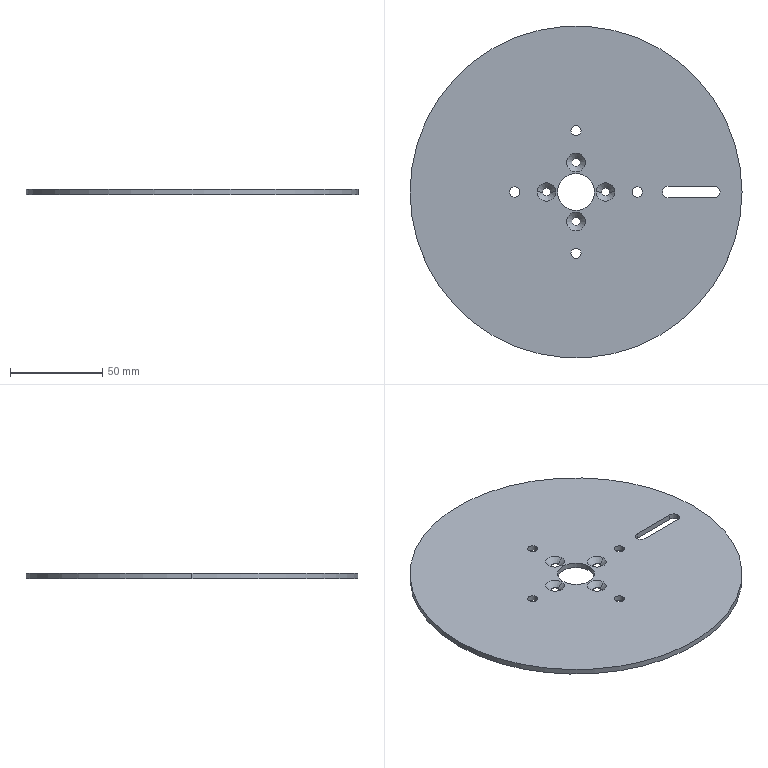Part | SolidWorks | features Chamfer 1, Extrusion 1, ICE 1 | 1 solid | 35 faces | box 180 x 180 x 3 mm | volume 74053 mm3 | cylinder 23 | cone 8 | plane 4 | commonest cylinder face diameters 4.5 x8 5.5 x8 6.2 x3 20 x2 180 x2
STEP:
#1=CARTESIAN_POINT('',(-18.25,0.,0.2));
#2=VERTEX_POINT('',#1);
#3=CARTESIAN_POINT('',(-13.75,0.,0.2));
#4=VERTEX_POINT('',#3);
#5=CARTESIAN_POINT('',(-16.,0.,0.2));
#6=DIRECTION('',(0.,0.,1.));
#7=DIRECTION('',(1.,0.,0.));
#8=AXIS2_PLACEMENT_3D('',#5,#6,#7);
#9=CIRCLE('',#8,2.25);
#10=EDGE_CURVE('',#2,#4,#9,.T.);
#11=ORIENTED_EDGE('',*,*,#10,.F.);
#12=CARTESIAN_POINT('',(-21.05,0.,3.));
#13=VERTEX_POINT('',#12);
#14=CARTESIAN_POINT('',(-18.25,0.,0.2));
#15=DIRECTION('',(-0.7071,0.,0.7071));
#16=VECTOR('',#15,1000.);
#17=LINE('',#14,#16);
#18=EDGE_CURVE('',#2,#13,#17,.T.);
#19=ORIENTED_EDGE('',*,*,#18,.T.);
#20=CARTESIAN_POINT('',(-10.95,0.,3.));
#21=VERTEX_POINT('',#20);
#22=CARTESIAN_POINT('',(-16.,0.,3.));
#23=DIRECTION('',(0.,0.,-1.));
#24=DIRECTION('',(1.,0.,0.));
#25=AXIS2_PLACEMENT_3D('',#22,#23,#24);
#26=CIRCLE('',#25,5.05);
#27=EDGE_CURVE('',#21,#13,#26,.T.);
#28=ORIENTED_EDGE('',*,*,#27,.F.);
#29=CARTESIAN_POINT('',(-13.75,0.,0.2));
#30=DIRECTION('',(0.7071,0.,0.7071));
#31=VECTOR('',#30,1000.);
#32=LINE('',#29,#31);
#33=EDGE_CURVE('',#4,#21,#32,.T.);
#34=ORIENTED_EDGE('',*,*,#33,.F.);
#35=EDGE_LOOP('',(#11,#19,#28,#34));
#36=FACE_OUTER_BOUND('',#35,.T.);
#37=CARTESIAN_POINT('',(-16.,0.,0.2));
#38=DIRECTION('',(0.,0.,1.));
#39=DIRECTION('',(1.,0.,0.));
#40=AXIS2_PLACEMENT_3D('',#37,#38,#39);
#41=CONICAL_SURFACE('',#40,2.25,0.7854);
#42=ADVANCED_FACE('',(#36),#41,.F.);
#43=CARTESIAN_POINT('',(-2.25,16.,0.2));
#44=VERTEX_POINT('',#43);
#45=CARTESIAN_POINT('',(2.25,16.,0.2));
#46=VERTEX_POINT('',#45);
#47=CARTESIAN_POINT('',(0.,16.,0.2));
#48=DIRECTION('',(0.,0.,1.));
#49=DIRECTION('',(1.,0.,0.));
#50=AXIS2_PLACEMENT_3D('',#47,#48,#49);
#51=CIRCLE('',#50,2.25);
#52=EDGE_CURVE('',#44,#46,#51,.T.);
#53=ORIENTED_EDGE('',*,*,#52,.F.);
#54=CARTESIAN_POINT('',(-5.05,16.,3.));
#55=VERTEX_POINT('',#54);
#56=CARTESIAN_POINT('',(-2.25,16.,0.2));
#57=DIRECTION('',(-0.7071,0.,0.7071));
#58=VECTOR('',#57,1000.);
#59=LINE('',#56,#58);
#60=EDGE_CURVE('',#44,#55,#59,.T.);
#61=ORIENTED_EDGE('',*,*,#60,.T.);
#62=CARTESIAN_POINT('',(5.05,16.,3.));
#63=VERTEX_POINT('',#62);
#64=CARTESIAN_POINT('',(0.,16.,3.));
#65=DIRECTION('',(0.,0.,-1.));
#66=DIRECTION('',(1.,0.,0.));
#67=AXIS2_PLACEMENT_3D('',#64,#65,#66);
#68=CIRCLE('',#67,5.05);
#69=EDGE_CURVE('',#63,#55,#68,.T.);
#70=ORIENTED_EDGE('',*,*,#69,.F.);
#71=CARTESIAN_POINT('',(2.25,16.,0.2));
#72=DIRECTION('',(0.7071,0.,0.7071));
#73=VECTOR('',#72,1000.);
#74=LINE('',#71,#73);
#75=EDGE_CURVE('',#46,#63,#74,.T.);
#76=ORIENTED_EDGE('',*,*,#75,.F.);
#77=EDGE_LOOP('',(#53,#61,#70,#76));
#78=FACE_OUTER_BOUND('',#77,.T.);
#79=CARTESIAN_POINT('',(0.,16.,0.2));
#80=DIRECTION('',(0.,0.,1.));
#81=DIRECTION('',(1.,0.,0.));
#82=AXIS2_PLACEMENT_3D('',#79,#80,#81);
#83=CONICAL_SURFACE('',#82,2.25,0.7854);
#84=ADVANCED_FACE('',(#78),#83,.F.);
#85=CARTESIAN_POINT('',(13.75,0.,0.2));
#86=VERTEX_POINT('',#85);
#87=CARTESIAN_POINT('',(18.25,0.,0.2));
#88=VERTEX_POINT('',#87);
#89=CARTESIAN_POINT('',(16.,0.,0.2));
#90=DIRECTION('',(0.,0.,1.));
#91=DIRECTION('',(1.,0.,0.));
#92=AXIS2_PLACEMENT_3D('',#89,#90,#91);
#93=CIRCLE('',#92,2.25);
#94=EDGE_CURVE('',#86,#88,#93,.T.);
#95=ORIENTED_EDGE('',*,*,#94,.F.);
#96=CARTESIAN_POINT('',(10.95,0.,3.));
#97=VERTEX_POINT('',#96);
#98=CARTESIAN_POINT('',(13.75,0.,0.2));
#99=DIRECTION('',(-0.7071,0.,0.7071));
#100=VECTOR('',#99,1000.);
#101=LINE('',#98,#100);
#102=EDGE_CURVE('',#86,#97,#101,.T.);
#103=ORIENTED_EDGE('',*,*,#102,.T.);
#104=CARTESIAN_POINT('',(21.05,0.,3.));
#105=VERTEX_POINT('',#104);
#106=CARTESIAN_POINT('',(16.,0.,3.));
#107=DIRECTION('',(0.,0.,-1.));
#108=DIRECTION('',(1.,0.,0.));
#109=AXIS2_PLACEMENT_3D('',#106,#107,#108);
#110=CIRCLE('',#109,5.05);
#111=EDGE_CURVE('',#105,#97,#110,.T.);
#112=ORIENTED_EDGE('',*,*,#111,.F.);
#113=CARTESIAN_POINT('',(18.25,0.,0.2));
#114=DIRECTION('',(0.7071,0.,0.7071));
#115=VECTOR('',#114,1000.);
#116=LINE('',#113,#115);
#117=EDGE_CURVE('',#88,#105,#116,.T.);
#118=ORIENTED_EDGE('',*,*,#117,.F.);
#119=EDGE_LOOP('',(#95,#103,#112,#118));
#120=FACE_OUTER_BOUND('',#119,.T.);
#121=CARTESIAN_POINT('',(16.,0.,0.2));
#122=DIRECTION('',(0.,0.,1.));
#123=DIRECTION('',(1.,0.,0.));
#124=AXIS2_PLACEMENT_3D('',#121,#122,#123);
#125=CONICAL_SURFACE('',#124,2.25,0.7854);
#126=ADVANCED_FACE('',(#120),#125,.F.);
#127=CARTESIAN_POINT('',(-2.25,-16.,0.2));
#128=VERTEX_POINT('',#127);
#129=CARTESIAN_POINT('',(2.25,-16.,0.2));
#130=VERTEX_POINT('',#129);
#131=CARTESIAN_POINT('',(0.,-16.,0.2));
#132=DIRECTION('',(0.,0.,1.));
#133=DIRECTION('',(1.,0.,0.));
#134=AXIS2_PLACEMENT_3D('',#131,#132,#133);
#135=CIRCLE('',#134,2.25);
#136=EDGE_CURVE('',#128,#130,#135,.T.);
#137=ORIENTED_EDGE('',*,*,#136,.F.);
#138=CARTESIAN_POINT('',(-5.05,-16.,3.));
#139=VERTEX_POINT('',#138);
#140=CARTESIAN_POINT('',(-2.25,-16.,0.2));
#141=DIRECTION('',(-0.7071,0.,0.7071));
#142=VECTOR('',#141,1000.);
#143=LINE('',#140,#142);
#144=EDGE_CURVE('',#128,#139,#143,.T.);
#145=ORIENTED_EDGE('',*,*,#144,.T.);
#146=CARTESIAN_POINT('',(5.05,-16.,3.));
#147=VERTEX_POINT('',#146);
#148=CARTESIAN_POINT('',(0.,-16.,3.));
#149=DIRECTION('',(0.,0.,-1.));
#150=DIRECTION('',(1.,0.,0.));
#151=AXIS2_PLACEMENT_3D('',#148,#149,#150);
#152=CIRCLE('',#151,5.05);
#153=EDGE_CURVE('',#147,#139,#152,.T.);
#154=ORIENTED_EDGE('',*,*,#153,.F.);
#155=CARTESIAN_POINT('',(2.25,-16.,0.2));
#156=DIRECTION('',(0.7071,0.,0.7071));
#157=VECTOR('',#156,1000.);
#158=LINE('',#155,#157);
#159=EDGE_CURVE('',#130,#147,#158,.T.);
#160=ORIENTED_EDGE('',*,*,#159,.F.);
#161=EDGE_LOOP('',(#137,#145,#154,#160));
#162=FACE_OUTER_BOUND('',#161,.T.);
#163=CARTESIAN_POINT('',(0.,-16.,0.2));
#164=DIRECTION('',(0.,0.,1.));
#165=DIRECTION('',(1.,0.,0.));
#166=AXIS2_PLACEMENT_3D('',#163,#164,#165);
#167=CONICAL_SURFACE('',#166,2.25,0.7854);
#168=ADVANCED_FACE('',(#162),#167,.F.);
#169=CARTESIAN_POINT('',(78.1,0.,0.));
#170=VERTEX_POINT('',#169);
#171=CARTESIAN_POINT('',(75.,3.1,0.));
#172=VERTEX_POINT('',#171);
#173=CARTESIAN_POINT('',(75.,0.,0.));
#174=DIRECTION('',(0.,0.,1.));
#175=DIRECTION('',(1.,0.,0.));
#176=AXIS2_PLACEMENT_3D('',#173,#174,#175);
#177=CIRCLE('',#176,3.1);
#178=EDGE_CURVE('',#170,#172,#177,.T.);
#179=ORIENTED_EDGE('',*,*,#178,.F.);
#180=CARTESIAN_POINT('',(78.1,0.,3.));
#181=VERTEX_POINT('',#180);
#182=CARTESIAN_POINT('',(78.1,0.,0.));
#183=DIRECTION('',(0.,0.,1.));
#184=VECTOR('',#183,1000.);
#185=LINE('',#182,#184);
#186=EDGE_CURVE('',#170,#181,#185,.T.);
#187=ORIENTED_EDGE('',*,*,#186,.T.);
#188=CARTESIAN_POINT('',(75.,3.1,3.));
#189=VERTEX_POINT('',#188);
#190=CARTESIAN_POINT('',(75.,0.,3.));
#191=DIRECTION('',(0.,0.,1.));
#192=DIRECTION('',(1.,0.,0.));
#193=AXIS2_PLACEMENT_3D('',#190,#191,#192);
#194=CIRCLE('',#193,3.1);
#195=EDGE_CURVE('',#181,#189,#194,.T.);
#196=ORIENTED_EDGE('',*,*,#195,.T.);
#197=CARTESIAN_POINT('',(75.,3.1,0.));
#198=DIRECTION('',(0.,0.,1.));
#199=VECTOR('',#198,1000.);
#200=LINE('',#197,#199);
#201=EDGE_CURVE('',#172,#189,#200,.T.);
#202=ORIENTED_EDGE('',*,*,#201,.F.);
#203=EDGE_LOOP('',(#179,#187,#196,#202));
#204=FACE_OUTER_BOUND('',#203,.T.);
#205=CARTESIAN_POINT('',(75.,0.,0.));
#206=DIRECTION('',(0.,0.,1.));
#207=DIRECTION('',(1.,0.,0.));
#208=AXIS2_PLACEMENT_3D('',#205,#206,#207);
#209=CYLINDRICAL_SURFACE('',#208,3.1);
#210=ADVANCED_FACE('',(#204),#209,.F.);
#211=CARTESIAN_POINT('',(30.5,0.,0.));
#212=VERTEX_POINT('',#211);
#213=CARTESIAN_POINT('',(36.,0.,0.));
#214=VERTEX_POINT('',#213);
#215=CARTESIAN_POINT('',(33.25,0.,0.));
#216=DIRECTION('',(0.,0.,1.));
#217=DIRECTION('',(1.,0.,0.));
#218=AXIS2_PLACEMENT_3D('',#215,#216,#217);
#219=CIRCLE('',#218,2.75);
#220=EDGE_CURVE('',#212,#214,#219,.T.);
#221=ORIENTED_EDGE('',*,*,#220,.F.);
#222=CARTESIAN_POINT('',(30.5,0.,3.));
#223=VERTEX_POINT('',#222);
#224=CARTESIAN_POINT('',(30.5,0.,0.));
#225=DIRECTION('',(0.,0.,1.));
#226=VECTOR('',#225,1000.);
#227=LINE('',#224,#226);
#228=EDGE_CURVE('',#212,#223,#227,.T.);
#229=ORIENTED_EDGE('',*,*,#228,.T.);
#230=CARTESIAN_POINT('',(36.,0.,3.));
#231=VERTEX_POINT('',#230);
#232=CARTESIAN_POINT('',(33.25,0.,3.));
#233=DIRECTION('',(0.,0.,1.));
#234=DIRECTION('',(1.,0.,0.));
#235=AXIS2_PLACEMENT_3D('',#232,#233,#234);
#236=CIRCLE('',#235,2.75);
#237=EDGE_CURVE('',#223,#231,#236,.T.);
#238=ORIENTED_EDGE('',*,*,#237,.T.);
#239=CARTESIAN_POINT('',(36.,0.,0.));
#240=DIRECTION('',(0.,0.,1.));
#241=VECTOR('',#240,1000.);
#242=LINE('',#239,#241);
#243=EDGE_CURVE('',#214,#231,#242,.T.);
#244=ORIENTED_EDGE('',*,*,#243,.F.);
#245=EDGE_LOOP('',(#221,#229,#238,#244));
#246=FACE_OUTER_BOUND('',#245,.T.);
#247=CARTESIAN_POINT('',(33.25,0.,0.));
#248=DIRECTION('',(0.,0.,1.));
#249=DIRECTION('',(1.,0.,0.));
#250=AXIS2_PLACEMENT_3D('',#247,#248,#249);
#251=CYLINDRICAL_SURFACE('',#250,2.75);
#252=ADVANCED_FACE('',(#246),#251,.F.);
#253=CARTESIAN_POINT('',(-2.75,-33.25,0.));
#254=VERTEX_POINT('',#253);
#255=CARTESIAN_POINT('',(2.75,-33.25,0.));
#256=VERTEX_POINT('',#255);
#257=CARTESIAN_POINT('',(0.,-33.25,0.));
#258=DIRECTION('',(0.,0.,1.));
#259=DIRECTION('',(1.,0.,0.));
#260=AXIS2_PLACEMENT_3D('',#257,#258,#259);
#261=CIRCLE('',#260,2.75);
#262=EDGE_CURVE('',#254,#256,#261,.T.);
#263=ORIENTED_EDGE('',*,*,#262,.F.);
#264=CARTESIAN_POINT('',(-2.75,-33.25,3.));
#265=VERTEX_POINT('',#264);
#266=CARTESIAN_POINT('',(-2.75,-33.25,0.));
#267=DIRECTION('',(0.,0.,1.));
#268=VECTOR('',#267,1000.);
#269=LINE('',#266,#268);
#270=EDGE_CURVE('',#254,#265,#269,.T.);
#271=ORIENTED_EDGE('',*,*,#270,.T.);
#272=CARTESIAN_POINT('',(2.75,-33.25,3.));
#273=VERTEX_POINT('',#272);
#274=CARTESIAN_POINT('',(0.,-33.25,3.));
#275=DIRECTION('',(0.,0.,1.));
#276=DIRECTION('',(1.,0.,0.));
#277=AXIS2_PLACEMENT_3D('',#274,#275,#276);
#278=CIRCLE('',#277,2.75);
#279=EDGE_CURVE('',#265,#273,#278,.T.);
#280=ORIENTED_EDGE('',*,*,#279,.T.);
#281=CARTESIAN_POINT('',(2.75,-33.25,0.));
#282=DIRECTION('',(0.,0.,1.));
#283=VECTOR('',#282,1000.);
#284=LINE('',#281,#283);
#285=EDGE_CURVE('',#256,#273,#284,.T.);
#286=ORIENTED_EDGE('',*,*,#285,.F.);
#287=EDGE_LOOP('',(#263,#271,#280,#286));
#288=FACE_OUTER_BOUND('',#287,.T.);
#289=CARTESIAN_POINT('',(0.,-33.25,0.));
#290=DIRECTION('',(0.,0.,1.));
#291=DIRECTION('',(1.,0.,0.));
#292=AXIS2_PLACEMENT_3D('',#289,#290,#291);
#293=CYLINDRICAL_SURFACE('',#292,2.75);
#294=ADVANCED_FACE('',(#288),#293,.F.);
#295=CARTESIAN_POINT('',(-36.,0.,0.));
#296=VERTEX_POINT('',#295);
#297=CARTESIAN_POINT('',(-30.5,0.,0.));
#298=VERTEX_POINT('',#297);
#299=CARTESIAN_POINT('',(-33.25,0.,0.));
#300=DIRECTION('',(0.,0.,1.));
#301=DIRECTION('',(1.,0.,0.));
#302=AXIS2_PLACEMENT_3D('',#299,#300,#301);
#303=CIRCLE('',#302,2.75);
#304=EDGE_CURVE('',#296,#298,#303,.T.);
#305=ORIENTED_EDGE('',*,*,#304,.F.);
#306=CARTESIAN_POINT('',(-36.,0.,3.));
#307=VERTEX_POINT('',#306);
#308=CARTESIAN_POINT('',(-36.,0.,0.));
#309=DIRECTION('',(0.,0.,1.));
#310=VECTOR('',#309,1000.);
#311=LINE('',#308,#310);
#312=EDGE_CURVE('',#296,#307,#311,.T.);
#313=ORIENTED_EDGE('',*,*,#312,.T.);
#314=CARTESIAN_POINT('',(-30.5,0.,3.));
#315=VERTEX_POINT('',#314);
#316=CARTESIAN_POINT('',(-33.25,0.,3.));
#317=DIRECTION('',(0.,0.,1.));
#318=DIRECTION('',(1.,0.,0.));
#319=AXIS2_PLACEMENT_3D('',#316,#317,#318);
#320=CIRCLE('',#319,2.75);
#321=EDGE_CURVE('',#307,#315,#320,.T.);
#322=ORIENTED_EDGE('',*,*,#321,.T.);
#323=CARTESIAN_POINT('',(-30.5,0.,0.));
#324=DIRECTION('',(0.,0.,1.));
#325=VECTOR('',#324,1000.);
#326=LINE('',#323,#325);
#327=EDGE_CURVE('',#298,#315,#326,.T.);
#328=ORIENTED_EDGE('',*,*,#327,.F.);
#329=EDGE_LOOP('',(#305,#313,#322,#328));
#330=FACE_OUTER_BOUND('',#329,.T.);
#331=CARTESIAN_POINT('',(-33.25,0.,0.));
#332=DIRECTION('',(0.,0.,1.));
#333=DIRECTION('',(1.,0.,0.));
#334=AXIS2_PLACEMENT_3D('',#331,#332,#333);
#335=CYLINDRICAL_SURFACE('',#334,2.75);
#336=ADVANCED_FACE('',(#330),#335,.F.);
#337=CARTESIAN_POINT('',(-2.75,33.25,0.));
#338=VERTEX_POINT('',#337);
#339=CARTESIAN_POINT('',(2.75,33.25,0.));
#340=VERTEX_POINT('',#339);
#341=CARTESIAN_POINT('',(0.,33.25,0.));
#342=DIRECTION('',(0.,0.,1.));
#343=DIRECTION('',(1.,0.,0.));
#344=AXIS2_PLACEMENT_3D('',#341,#342,#343);
#345=CIRCLE('',#344,2.75);
#346=EDGE_CURVE('',#338,#340,#345,.T.);
#347=ORIENTED_EDGE('',*,*,#346,.F.);
#348=CARTESIAN_POINT('',(-2.75,33.25,3.));
#349=VERTEX_POINT('',#348);
#350=CARTESIAN_POINT('',(-2.75,33.25,0.));
#351=DIRECTION('',(0.,0.,1.));
#352=VECTOR('',#351,1000.);
#353=LINE('',#350,#352);
#354=EDGE_CURVE('',#338,#349,#353,.T.);
#355=ORIENTED_EDGE('',*,*,#354,.T.);
#356=CARTESIAN_POINT('',(2.75,33.25,3.));
#357=VERTEX_POINT('',#356);
#358=CARTESIAN_POINT('',(0.,33.25,3.));
#359=DIRECTION('',(0.,0.,1.));
#360=DIRECTION('',(1.,0.,0.));
#361=AXIS2_PLACEMENT_3D('',#358,#359,#360);
#362=CIRCLE('',#361,2.75);
#363=EDGE_CURVE('',#349,#357,#362,.T.);
#364=ORIENTED_EDGE('',*,*,#363,.T.);
#365=CARTESIAN_POINT('',(2.75,33.25,0.));
#366=DIRECTION('',(0.,0.,1.));
#367=VECTOR('',#366,1000.);
#368=LINE('',#365,#367);
#369=EDGE_CURVE('',#340,#357,#368,.T.);
#370=ORIENTED_EDGE('',*,*,#369,.F.);
#371=EDGE_LOOP('',(#347,#355,#364,#370));
#372=FACE_OUTER_BOUND('',#371,.T.);
#373=CARTESIAN_POINT('',(0.,33.25,0.));
#374=DIRECTION('',(0.,0.,1.));
#375=DIRECTION('',(1.,0.,0.));
#376=AXIS2_PLACEMENT_3D('',#373,#374,#375);
#377=CYLINDRICAL_SURFACE('',#376,2.75);
#378=ADVANCED_FACE('',(#372),#377,.F.);
#379=CARTESIAN_POINT('',(13.75,0.,0.));
#380=VERTEX_POINT('',#379);
#381=CARTESIAN_POINT('',(18.25,0.,0.));
#382=VERTEX_POINT('',#381);
#383=CARTESIAN_POINT('',(16.,0.,0.));
#384=DIRECTION('',(0.,0.,1.));
#385=DIRECTION('',(1.,0.,0.));
#386=AXIS2_PLACEMENT_3D('',#383,#384,#385);
#387=CIRCLE('',#386,2.25);
#388=EDGE_CURVE('',#380,#382,#387,.T.);
#389=ORIENTED_EDGE('',*,*,#388,.F.);
#390=CARTESIAN_POINT('',(13.75,0.,0.));
#391=DIRECTION('',(0.,0.,1.));
#392=VECTOR('',#391,1000.);
#393=LINE('',#390,#392);
#394=EDGE_CURVE('',#380,#86,#393,.T.);
#395=ORIENTED_EDGE('',*,*,#394,.T.);
#396=ORIENTED_EDGE('',*,*,#94,.T.);
#397=CARTESIAN_POINT('',(18.25,0.,0.));
#398=DIRECTION('',(0.,0.,1.));
#399=VECTOR('',#398,1000.);
#400=LINE('',#397,#399);
#401=EDGE_CURVE('',#382,#88,#400,.T.);
#402=ORIENTED_EDGE('',*,*,#401,.F.);
#403=EDGE_LOOP('',(#389,#395,#396,#402));
#404=FACE_OUTER_BOUND('',#403,.T.);
#405=CARTESIAN_POINT('',(16.,0.,0.));
#406=DIRECTION('',(0.,0.,1.));
#407=DIRECTION('',(1.,0.,0.));
#408=AXIS2_PLACEMENT_3D('',#405,#406,#407);
#409=CYLINDRICAL_SURFACE('',#408,2.25);
#410=ADVANCED_FACE('',(#404),#409,.F.);
#411=CARTESIAN_POINT('',(-2.25,-16.,0.));
#412=VERTEX_POINT('',#411);
#413=CARTESIAN_POINT('',(2.25,-16.,0.));
#414=VERTEX_POINT('',#413);
#415=CARTESIAN_POINT('',(0.,-16.,0.));
#416=DIRECTION('',(0.,0.,1.));
#417=DIRECTION('',(1.,0.,0.));
#418=AXIS2_PLACEMENT_3D('',#415,#416,#417);
#419=CIRCLE('',#418,2.25);
#420=EDGE_CURVE('',#412,#414,#419,.T.);
#421=ORIENTED_EDGE('',*,*,#420,.F.);
#422=CARTESIAN_POINT('',(-2.25,-16.,0.));
#423=DIRECTION('',(0.,0.,1.));
#424=VECTOR('',#423,1000.);
#425=LINE('',#422,#424);
#426=EDGE_CURVE('',#412,#128,#425,.T.);
#427=ORIENTED_EDGE('',*,*,#426,.T.);
#428=ORIENTED_EDGE('',*,*,#136,.T.);
#429=CARTESIAN_POINT('',(2.25,-16.,0.));
#430=DIRECTION('',(0.,0.,1.));
#431=VECTOR('',#430,1000.);
#432=LINE('',#429,#431);
#433=EDGE_CURVE('',#414,#130,#432,.T.);
#434=ORIENTED_EDGE('',*,*,#433,.F.);
#435=EDGE_LOOP('',(#421,#427,#428,#434));
#436=FACE_OUTER_BOUND('',#435,.T.);
#437=CARTESIAN_POINT('',(0.,-16.,0.));
#438=DIRECTION('',(0.,0.,1.));
#439=DIRECTION('',(1.,0.,0.));
#440=AXIS2_PLACEMENT_3D('',#437,#438,#439);
#441=CYLINDRICAL_SURFACE('',#440,2.25);
#442=ADVANCED_FACE('',(#436),#441,.F.);
#443=CARTESIAN_POINT('',(-18.25,0.,0.));
#444=VERTEX_POINT('',#443);
#445=CARTESIAN_POINT('',(-13.75,0.,0.));
#446=VERTEX_POINT('',#445);
#447=CARTESIAN_POINT('',(-16.,0.,0.));
#448=DIRECTION('',(0.,0.,1.));
#449=DIRECTION('',(1.,0.,0.));
#450=AXIS2_PLACEMENT_3D('',#447,#448,#449);
#451=CIRCLE('',#450,2.25);
#452=EDGE_CURVE('',#444,#446,#451,.T.);
#453=ORIENTED_EDGE('',*,*,#452,.F.);
#454=CARTESIAN_POINT('',(-18.25,0.,0.));
#455=DIRECTION('',(0.,0.,1.));
#456=VECTOR('',#455,1000.);
#457=LINE('',#454,#456);
#458=EDGE_CURVE('',#444,#2,#457,.T.);
#459=ORIENTED_EDGE('',*,*,#458,.T.);
#460=ORIENTED_EDGE('',*,*,#10,.T.);
#461=CARTESIAN_POINT('',(-13.75,0.,0.));
#462=DIRECTION('',(0.,0.,1.));
#463=VECTOR('',#462,1000.);
#464=LINE('',#461,#463);
#465=EDGE_CURVE('',#446,#4,#464,.T.);
#466=ORIENTED_EDGE('',*,*,#465,.F.);
#467=EDGE_LOOP('',(#453,#459,#460,#466));
#468=FACE_OUTER_BOUND('',#467,.T.);
#469=CARTESIAN_POINT('',(-16.,0.,0.));
#470=DIRECTION('',(0.,0.,1.));
#471=DIRECTION('',(1.,0.,0.));
#472=AXIS2_PLACEMENT_3D('',#469,#470,#471);
#473=CYLINDRICAL_SURFACE('',#472,2.25);
#474=ADVANCED_FACE('',(#468),#473,.F.);
#475=CARTESIAN_POINT('',(-2.25,16.,0.));
#476=VERTEX_POINT('',#475);
#477=CARTESIAN_POINT('',(2.25,16.,0.));
#478=VERTEX_POINT('',#477);
#479=CARTESIAN_POINT('',(0.,16.,0.));
#480=DIRECTION('',(0.,0.,1.));
#481=DIRECTION('',(1.,0.,0.));
#482=AXIS2_PLACEMENT_3D('',#479,#480,#481);
#483=CIRCLE('',#482,2.25);
#484=EDGE_CURVE('',#476,#478,#483,.T.);
#485=ORIENTED_EDGE('',*,*,#484,.F.);
#486=CARTESIAN_POINT('',(-2.25,16.,0.));
#487=DIRECTION('',(0.,0.,1.));
#488=VECTOR('',#487,1000.);
#489=LINE('',#486,#488);
#490=EDGE_CURVE('',#476,#44,#489,.T.);
#491=ORIENTED_EDGE('',*,*,#490,.T.);
#492=ORIENTED_EDGE('',*,*,#52,.T.);
#493=CARTESIAN_POINT('',(2.25,16.,0.));
#494=DIRECTION('',(0.,0.,1.));
#495=VECTOR('',#494,1000.);
#496=LINE('',#493,#495);
#497=EDGE_CURVE('',#478,#46,#496,.T.);
#498=ORIENTED_EDGE('',*,*,#497,.F.);
#499=EDGE_LOOP('',(#485,#491,#492,#498));
#500=FACE_OUTER_BOUND('',#499,.T.);
#501=CARTESIAN_POINT('',(0.,16.,0.));
#502=DIRECTION('',(0.,0.,1.));
#503=DIRECTION('',(1.,0.,0.));
#504=AXIS2_PLACEMENT_3D('',#501,#502,#503);
#505=CYLINDRICAL_SURFACE('',#504,2.25);
#506=ADVANCED_FACE('',(#500),#505,.F.);
#507=CARTESIAN_POINT('',(-10.,0.,3.));
#508=VERTEX_POINT('',#507);
#509=CARTESIAN_POINT('',(10.,0.,3.));
#510=VERTEX_POINT('',#509);
#511=CARTESIAN_POINT('',(0.,0.,3.));
#512=DIRECTION('',(0.,0.,1.));
#513=DIRECTION('',(1.,0.,0.));
#514=AXIS2_PLACEMENT_3D('',#511,#512,#513);
#515=CIRCLE('',#514,10.);
#516=EDGE_CURVE('',#508,#510,#515,.T.);
#517=ORIENTED_EDGE('',*,*,#516,.T.);
#518=CARTESIAN_POINT('',(10.,0.,0.));
#519=VERTEX_POINT('',#518);
#520=CARTESIAN_POINT('',(10.,0.,3.));
#521=DIRECTION('',(0.,0.,-1.));
#522=VECTOR('',#521,1000.);
#523=LINE('',#520,#522);
#524=EDGE_CURVE('',#510,#519,#523,.T.);
#525=ORIENTED_EDGE('',*,*,#524,.T.);
#526=CARTESIAN_POINT('',(-10.,0.,0.));
#527=VERTEX_POINT('',#526);
#528=CARTESIAN_POINT('',(0.,0.,0.));
#529=DIRECTION('',(0.,0.,1.));
#530=DIRECTION('',(1.,0.,0.));
#531=AXIS2_PLACEMENT_3D('',#528,#529,#530);
#532=CIRCLE('',#531,10.);
#533=EDGE_CURVE('',#527,#519,#532,.T.);
#534=ORIENTED_EDGE('',*,*,#533,.F.);
#535=CARTESIAN_POINT('',(-10.,0.,3.));
#536=DIRECTION('',(0.,0.,-1.));
#537=VECTOR('',#536,1000.);
#538=LINE('',#535,#537);
#539=EDGE_CURVE('',#508,#527,#538,.T.);
#540=ORIENTED_EDGE('',*,*,#539,.F.);
#541=EDGE_LOOP('',(#517,#525,#534,#540));
#542=FACE_OUTER_BOUND('',#541,.T.);
#543=CARTESIAN_POINT('',(0.,0.,3.));
#544=DIRECTION('',(0.,0.,-1.));
#545=DIRECTION('',(-1.,0.,0.));
#546=AXIS2_PLACEMENT_3D('',#543,#544,#545);
#547=CYLINDRICAL_SURFACE('',#546,10.);
#548=ADVANCED_FACE('',(#542),#547,.F.);
#549=CARTESIAN_POINT('',(90.,0.,3.));
#550=VERTEX_POINT('',#549);
#551=CARTESIAN_POINT('',(-90.,0.,3.));
#552=VERTEX_POINT('',#551);
#553=CARTESIAN_POINT('',(0.,0.,3.));
#554=DIRECTION('',(0.,0.,1.));
#555=DIRECTION('',(1.,0.,0.));
#556=AXIS2_PLACEMENT_3D('',#553,#554,#555);
#557=CIRCLE('',#556,90.);
#558=EDGE_CURVE('',#550,#552,#557,.T.);
#559=ORIENTED_EDGE('',*,*,#558,.F.);
#560=CARTESIAN_POINT('',(90.,0.,0.));
#561=VERTEX_POINT('',#560);
#562=CARTESIAN_POINT('',(90.,0.,3.));
#563=DIRECTION('',(0.,0.,-1.));
#564=VECTOR('',#563,1000.);
#565=LINE('',#562,#564);
#566=EDGE_CURVE('',#550,#561,#565,.T.);
#567=ORIENTED_EDGE('',*,*,#566,.T.);
#568=CARTESIAN_POINT('',(-90.,0.,0.));
#569=VERTEX_POINT('',#568);
#570=CARTESIAN_POINT('',(0.,0.,0.));
#571=DIRECTION('',(0.,0.,1.));
#572=DIRECTION('',(1.,0.,0.));
#573=AXIS2_PLACEMENT_3D('',#570,#571,#572);
#574=CIRCLE('',#573,90.);
#575=EDGE_CURVE('',#561,#569,#574,.T.);
#576=ORIENTED_EDGE('',*,*,#575,.T.);
#577=CARTESIAN_POINT('',(-90.,0.,3.));
#578=DIRECTION('',(0.,0.,-1.));
#579=VECTOR('',#578,1000.);
#580=LINE('',#577,#579);
#581=EDGE_CURVE('',#552,#569,#580,.T.);
#582=ORIENTED_EDGE('',*,*,#581,.F.);
#583=EDGE_LOOP('',(#559,#567,#576,#582));
#584=FACE_OUTER_BOUND('',#583,.T.);
#585=CARTESIAN_POINT('',(0.,0.,3.));
#586=DIRECTION('',(0.,0.,-1.));
#587=DIRECTION('',(-1.,0.,0.));
#588=AXIS2_PLACEMENT_3D('',#585,#586,#587);
#589=CYLINDRICAL_SURFACE('',#588,90.);
#590=ADVANCED_FACE('',(#584),#589,.T.);
#591=ORIENTED_EDGE('',*,*,#153,.T.);
#592=CARTESIAN_POINT('',(0.,-16.,3.));
#593=DIRECTION('',(0.,0.,-1.));
#594=DIRECTION('',(1.,0.,0.));
#595=AXIS2_PLACEMENT_3D('',#592,#593,#594);
#596=CIRCLE('',#595,5.05);
#597=EDGE_CURVE('',#139,#147,#596,.T.);
#598=ORIENTED_EDGE('',*,*,#597,.T.);
#599=EDGE_LOOP('',(#591,#598));
#600=FACE_BOUND('',#599,.T.);
#601=ORIENTED_EDGE('',*,*,#111,.T.);
#602=CARTESIAN_POINT('',(16.,0.,3.));
#603=DIRECTION('',(0.,0.,-1.));
#604=DIRECTION('',(1.,0.,0.));
#605=AXIS2_PLACEMENT_3D('',#602,#603,#604);
#606=CIRCLE('',#605,5.05);
#607=EDGE_CURVE('',#97,#105,#606,.T.);
#608=ORIENTED_EDGE('',*,*,#607,.T.);
#609=EDGE_LOOP('',(#601,#608));
#610=FACE_BOUND('',#609,.T.);
#611=ORIENTED_EDGE('',*,*,#69,.T.);
#612=CARTESIAN_POINT('',(0.,16.,3.));
#613=DIRECTION('',(0.,0.,-1.));
#614=DIRECTION('',(1.,0.,0.));
#615=AXIS2_PLACEMENT_3D('',#612,#613,#614);
#616=CIRCLE('',#615,5.05);
#617=EDGE_CURVE('',#55,#63,#616,.T.);
#618=ORIENTED_EDGE('',*,*,#617,.T.);
#619=EDGE_LOOP('',(#611,#618));
#620=FACE_BOUND('',#619,.T.);
#621=ORIENTED_EDGE('',*,*,#27,.T.);
#622=CARTESIAN_POINT('',(-16.,0.,3.));
#623=DIRECTION('',(0.,0.,-1.));
#624=DIRECTION('',(1.,0.,0.));
#625=AXIS2_PLACEMENT_3D('',#622,#623,#624);
#626=CIRCLE('',#625,5.05);
#627=EDGE_CURVE('',#13,#21,#626,.T.);
#628=ORIENTED_EDGE('',*,*,#627,.T.);
#629=EDGE_LOOP('',(#621,#628));
#630=FACE_BOUND('',#629,.T.);
#631=CARTESIAN_POINT('',(50.,3.1,3.));
#632=VERTEX_POINT('',#631);
#633=CARTESIAN_POINT('',(50.,-3.1,3.));
#634=VERTEX_POINT('',#633);
#635=CARTESIAN_POINT('',(50.,0.,3.));
#636=DIRECTION('',(0.,0.,1.));
#637=DIRECTION('',(1.,0.,0.));
#638=AXIS2_PLACEMENT_3D('',#635,#636,#637);
#639=CIRCLE('',#638,3.1);
#640=EDGE_CURVE('',#632,#634,#639,.T.);
#641=ORIENTED_EDGE('',*,*,#640,.F.);
#642=CARTESIAN_POINT('',(50.,3.1,3.));
#643=DIRECTION('',(-1.,0.,0.));
#644=VECTOR('',#643,1000.);
#645=LINE('',#642,#644);
#646=EDGE_CURVE('',#189,#632,#645,.T.);
#647=ORIENTED_EDGE('',*,*,#646,.F.);
#648=ORIENTED_EDGE('',*,*,#195,.F.);
#649=CARTESIAN_POINT('',(75.,-3.1,3.));
#650=VERTEX_POINT('',#649);
#651=CARTESIAN_POINT('',(75.,0.,3.));
#652=DIRECTION('',(0.,0.,1.));
#653=DIRECTION('',(1.,0.,0.));
#654=AXIS2_PLACEMENT_3D('',#651,#652,#653);
#655=CIRCLE('',#654,3.1);
#656=EDGE_CURVE('',#650,#181,#655,.T.);
#657=ORIENTED_EDGE('',*,*,#656,.F.);
#658=CARTESIAN_POINT('',(50.,-3.1,3.));
#659=DIRECTION('',(1.,0.,0.));
#660=VECTOR('',#659,1000.);
#661=LINE('',#658,#660);
#662=EDGE_CURVE('',#634,#650,#661,.T.);
#663=ORIENTED_EDGE('',*,*,#662,.F.);
#664=EDGE_LOOP('',(#641,#647,#648,#657,#663));
#665=FACE_BOUND('',#664,.T.);
#666=CARTESIAN_POINT('',(33.25,0.,3.));
#667=DIRECTION('',(0.,0.,1.));
#668=DIRECTION('',(1.,0.,0.));
#669=AXIS2_PLACEMENT_3D('',#666,#667,#668);
#670=CIRCLE('',#669,2.75);
#671=EDGE_CURVE('',#231,#223,#670,.T.);
#672=ORIENTED_EDGE('',*,*,#671,.F.);
#673=ORIENTED_EDGE('',*,*,#237,.F.);
#674=EDGE_LOOP('',(#672,#673));
#675=FACE_BOUND('',#674,.T.);
#676=CARTESIAN_POINT('',(0.,-33.25,3.));
#677=DIRECTION('',(0.,0.,1.));
#678=DIRECTION('',(1.,0.,0.));
#679=AXIS2_PLACEMENT_3D('',#676,#677,#678);
#680=CIRCLE('',#679,2.75);
#681=EDGE_CURVE('',#273,#265,#680,.T.);
#682=ORIENTED_EDGE('',*,*,#681,.F.);
#683=ORIENTED_EDGE('',*,*,#279,.F.);
#684=EDGE_LOOP('',(#682,#683));
#685=FACE_BOUND('',#684,.T.);
#686=CARTESIAN_POINT('',(-33.25,0.,3.));
#687=DIRECTION('',(0.,0.,1.));
#688=DIRECTION('',(1.,0.,0.));
#689=AXIS2_PLACEMENT_3D('',#686,#687,#688);
#690=CIRCLE('',#689,2.75);
#691=EDGE_CURVE('',#315,#307,#690,.T.);
#692=ORIENTED_EDGE('',*,*,#691,.F.);
#693=ORIENTED_EDGE('',*,*,#321,.F.);
#694=EDGE_LOOP('',(#692,#693));
#695=FACE_BOUND('',#694,.T.);
#696=CARTESIAN_POINT('',(0.,33.25,3.));
#697=DIRECTION('',(0.,0.,1.));
#698=DIRECTION('',(1.,0.,0.));
#699=AXIS2_PLACEMENT_3D('',#696,#697,#698);
#700=CIRCLE('',#699,2.75);
#701=EDGE_CURVE('',#357,#349,#700,.T.);
#702=ORIENTED_EDGE('',*,*,#701,.F.);
#703=ORIENTED_EDGE('',*,*,#363,.F.);
#704=EDGE_LOOP('',(#702,#703));
#705=FACE_BOUND('',#704,.T.);
#706=CARTESIAN_POINT('',(0.,0.,3.));
#707=DIRECTION('',(0.,0.,1.));
#708=DIRECTION('',(1.,0.,0.));
#709=AXIS2_PLACEMENT_3D('',#706,#707,#708);
#710=CIRCLE('',#709,90.);
#711=EDGE_CURVE('',#552,#550,#710,.T.);
#712=ORIENTED_EDGE('',*,*,#711,.T.);
#713=ORIENTED_EDGE('',*,*,#558,.T.);
#714=EDGE_LOOP('',(#712,#713));
#715=FACE_OUTER_BOUND('',#714,.T.);
#716=ORIENTED_EDGE('',*,*,#516,.F.);
#717=CARTESIAN_POINT('',(0.,0.,3.));
#718=DIRECTION('',(0.,0.,1.));
#719=DIRECTION('',(1.,0.,0.));
#720=AXIS2_PLACEMENT_3D('',#717,#718,#719);
#721=CIRCLE('',#720,10.);
#722=EDGE_CURVE('',#510,#508,#721,.T.);
#723=ORIENTED_EDGE('',*,*,#722,.F.);
#724=EDGE_LOOP('',(#716,#723));
#725=FACE_BOUND('',#724,.T.);
#726=CARTESIAN_POINT('',(0.,0.,3.));
#727=DIRECTION('',(0.,0.,1.));
#728=DIRECTION('',(1.,0.,0.));
#729=AXIS2_PLACEMENT_3D('',#726,#727,#728);
#730=PLANE('',#729);
#731=ADVANCED_FACE('',(#600,#610,#620,#630,#665,#675,#685,#695,#705,#715,#725),#730,.T.);
#732=CARTESIAN_POINT('',(50.,3.1,0.));
#733=VERTEX_POINT('',#732);
#734=CARTESIAN_POINT('',(50.,3.1,0.));
#735=DIRECTION('',(-1.,0.,0.));
#736=VECTOR('',#735,1000.);
#737=LINE('',#734,#736);
#738=EDGE_CURVE('',#172,#733,#737,.T.);
#739=ORIENTED_EDGE('',*,*,#738,.T.);
#740=CARTESIAN_POINT('',(50.,-3.1,0.));
#741=VERTEX_POINT('',#740);
#742=CARTESIAN_POINT('',(50.,0.,0.));
#743=DIRECTION('',(0.,0.,1.));
#744=DIRECTION('',(1.,0.,0.));
#745=AXIS2_PLACEMENT_3D('',#742,#743,#744);
#746=CIRCLE('',#745,3.1);
#747=EDGE_CURVE('',#733,#741,#746,.T.);
#748=ORIENTED_EDGE('',*,*,#747,.T.);
#749=CARTESIAN_POINT('',(75.,-3.1,0.));
#750=VERTEX_POINT('',#749);
#751=CARTESIAN_POINT('',(50.,-3.1,0.));
#752=DIRECTION('',(1.,0.,0.));
#753=VECTOR('',#752,1000.);
#754=LINE('',#751,#753);
#755=EDGE_CURVE('',#741,#750,#754,.T.);
#756=ORIENTED_EDGE('',*,*,#755,.T.);
#757=CARTESIAN_POINT('',(75.,0.,0.));
#758=DIRECTION('',(0.,0.,1.));
#759=DIRECTION('',(1.,0.,0.));
#760=AXIS2_PLACEMENT_3D('',#757,#758,#759);
#761=CIRCLE('',#760,3.1);
#762=EDGE_CURVE('',#750,#170,#761,.T.);
#763=ORIENTED_EDGE('',*,*,#762,.T.);
#764=ORIENTED_EDGE('',*,*,#178,.T.);
#765=EDGE_LOOP('',(#739,#748,#756,#763,#764));
#766=FACE_BOUND('',#765,.T.);
#767=CARTESIAN_POINT('',(33.25,0.,0.));
#768=DIRECTION('',(0.,0.,1.));
#769=DIRECTION('',(1.,0.,0.));
#770=AXIS2_PLACEMENT_3D('',#767,#768,#769);
#771=CIRCLE('',#770,2.75);
#772=EDGE_CURVE('',#214,#212,#771,.T.);
#773=ORIENTED_EDGE('',*,*,#772,.T.);
#774=ORIENTED_EDGE('',*,*,#220,.T.);
#775=EDGE_LOOP('',(#773,#774));
#776=FACE_BOUND('',#775,.T.);
#777=CARTESIAN_POINT('',(0.,-33.25,0.));
#778=DIRECTION('',(0.,0.,1.));
#779=DIRECTION('',(1.,0.,0.));
#780=AXIS2_PLACEMENT_3D('',#777,#778,#779);
#781=CIRCLE('',#780,2.75);
#782=EDGE_CURVE('',#256,#254,#781,.T.);
#783=ORIENTED_EDGE('',*,*,#782,.T.);
#784=ORIENTED_EDGE('',*,*,#262,.T.);
#785=EDGE_LOOP('',(#783,#784));
#786=FACE_BOUND('',#785,.T.);
#787=CARTESIAN_POINT('',(-33.25,0.,0.));
#788=DIRECTION('',(0.,0.,1.));
#789=DIRECTION('',(1.,0.,0.));
#790=AXIS2_PLACEMENT_3D('',#787,#788,#789);
#791=CIRCLE('',#790,2.75);
#792=EDGE_CURVE('',#298,#296,#791,.T.);
#793=ORIENTED_EDGE('',*,*,#792,.T.);
#794=ORIENTED_EDGE('',*,*,#304,.T.);
#795=EDGE_LOOP('',(#793,#794));
#796=FACE_BOUND('',#795,.T.);
#797=CARTESIAN_POINT('',(0.,33.25,0.));
#798=DIRECTION('',(0.,0.,1.));
#799=DIRECTION('',(1.,0.,0.));
#800=AXIS2_PLACEMENT_3D('',#797,#798,#799);
#801=CIRCLE('',#800,2.75);
#802=EDGE_CURVE('',#340,#338,#801,.T.);
#803=ORIENTED_EDGE('',*,*,#802,.T.);
#804=ORIENTED_EDGE('',*,*,#346,.T.);
#805=EDGE_LOOP('',(#803,#804));
#806=FACE_BOUND('',#805,.T.);
#807=CARTESIAN_POINT('',(16.,0.,0.));
#808=DIRECTION('',(0.,0.,1.));
#809=DIRECTION('',(1.,0.,0.));
#810=AXIS2_PLACEMENT_3D('',#807,#808,#809);
#811=CIRCLE('',#810,2.25);
#812=EDGE_CURVE('',#382,#380,#811,.T.);
#813=ORIENTED_EDGE('',*,*,#812,.T.);
#814=ORIENTED_EDGE('',*,*,#388,.T.);
#815=EDGE_LOOP('',(#813,#814));
#816=FACE_BOUND('',#815,.T.);
#817=CARTESIAN_POINT('',(0.,-16.,0.));
#818=DIRECTION('',(0.,0.,1.));
#819=DIRECTION('',(1.,0.,0.));
#820=AXIS2_PLACEMENT_3D('',#817,#818,#819);
#821=CIRCLE('',#820,2.25);
#822=EDGE_CURVE('',#414,#412,#821,.T.);
#823=ORIENTED_EDGE('',*,*,#822,.T.);
#824=ORIENTED_EDGE('',*,*,#420,.T.);
#825=EDGE_LOOP('',(#823,#824));
#826=FACE_BOUND('',#825,.T.);
#827=CARTESIAN_POINT('',(-16.,0.,0.));
#828=DIRECTION('',(0.,0.,1.));
#829=DIRECTION('',(1.,0.,0.));
#830=AXIS2_PLACEMENT_3D('',#827,#828,#829);
#831=CIRCLE('',#830,2.25);
#832=EDGE_CURVE('',#446,#444,#831,.T.);
#833=ORIENTED_EDGE('',*,*,#832,.T.);
#834=ORIENTED_EDGE('',*,*,#452,.T.);
#835=EDGE_LOOP('',(#833,#834));
#836=FACE_BOUND('',#835,.T.);
#837=CARTESIAN_POINT('',(0.,16.,0.));
#838=DIRECTION('',(0.,0.,1.));
#839=DIRECTION('',(1.,0.,0.));
#840=AXIS2_PLACEMENT_3D('',#837,#838,#839);
#841=CIRCLE('',#840,2.25);
#842=EDGE_CURVE('',#478,#476,#841,.T.);
#843=ORIENTED_EDGE('',*,*,#842,.T.);
#844=ORIENTED_EDGE('',*,*,#484,.T.);
#845=EDGE_LOOP('',(#843,#844));
#846=FACE_BOUND('',#845,.T.);
#847=CARTESIAN_POINT('',(0.,0.,0.));
#848=DIRECTION('',(0.,0.,1.));
#849=DIRECTION('',(1.,0.,0.));
#850=AXIS2_PLACEMENT_3D('',#847,#848,#849);
#851=CIRCLE('',#850,90.);
#852=EDGE_CURVE('',#569,#561,#851,.T.);
#853=ORIENTED_EDGE('',*,*,#852,.F.);
#854=ORIENTED_EDGE('',*,*,#575,.F.);
#855=EDGE_LOOP('',(#853,#854));
#856=FACE_OUTER_BOUND('',#855,.T.);
#857=ORIENTED_EDGE('',*,*,#533,.T.);
#858=CARTESIAN_POINT('',(0.,0.,0.));
#859=DIRECTION('',(0.,0.,1.));
#860=DIRECTION('',(1.,0.,0.));
#861=AXIS2_PLACEMENT_3D('',#858,#859,#860);
#862=CIRCLE('',#861,10.);
#863=EDGE_CURVE('',#519,#527,#862,.T.);
#864=ORIENTED_EDGE('',*,*,#863,.T.);
#865=EDGE_LOOP('',(#857,#864));
#866=FACE_BOUND('',#865,.T.);
#867=CARTESIAN_POINT('',(0.,0.,0.));
#868=DIRECTION('',(0.,0.,1.));
#869=DIRECTION('',(1.,0.,0.));
#870=AXIS2_PLACEMENT_3D('',#867,#868,#869);
#871=PLANE('',#870);
#872=ADVANCED_FACE('',(#766,#776,#786,#796,#806,#816,#826,#836,#846,#856,#866),#871,.F.);
#873=ORIENTED_EDGE('',*,*,#566,.F.);
#874=ORIENTED_EDGE('',*,*,#711,.F.);
#875=ORIENTED_EDGE('',*,*,#581,.T.);
#876=ORIENTED_EDGE('',*,*,#852,.T.);
#877=EDGE_LOOP('',(#873,#874,#875,#876));
#878=FACE_OUTER_BOUND('',#877,.T.);
#879=CARTESIAN_POINT('',(0.,0.,3.));
#880=DIRECTION('',(0.,0.,-1.));
#881=DIRECTION('',(-1.,0.,0.));
#882=AXIS2_PLACEMENT_3D('',#879,#880,#881);
#883=CYLINDRICAL_SURFACE('',#882,90.);
#884=ADVANCED_FACE('',(#878),#883,.T.);
#885=ORIENTED_EDGE('',*,*,#524,.F.);
#886=ORIENTED_EDGE('',*,*,#722,.T.);
#887=ORIENTED_EDGE('',*,*,#539,.T.);
#888=ORIENTED_EDGE('',*,*,#863,.F.);
#889=EDGE_LOOP('',(#885,#886,#887,#888));
#890=FACE_OUTER_BOUND('',#889,.T.);
#891=CARTESIAN_POINT('',(0.,0.,3.));
#892=DIRECTION('',(0.,0.,-1.));
#893=DIRECTION('',(-1.,0.,0.));
#894=AXIS2_PLACEMENT_3D('',#891,#892,#893);
#895=CYLINDRICAL_SURFACE('',#894,10.);
#896=ADVANCED_FACE('',(#890),#895,.F.);
#897=ORIENTED_EDGE('',*,*,#490,.F.);
#898=ORIENTED_EDGE('',*,*,#842,.F.);
#899=ORIENTED_EDGE('',*,*,#497,.T.);
#900=CARTESIAN_POINT('',(0.,16.,0.2));
#901=DIRECTION('',(0.,0.,1.));
#902=DIRECTION('',(1.,0.,0.));
#903=AXIS2_PLACEMENT_3D('',#900,#901,#902);
#904=CIRCLE('',#903,2.25);
#905=EDGE_CURVE('',#46,#44,#904,.T.);
#906=ORIENTED_EDGE('',*,*,#905,.T.);
#907=EDGE_LOOP('',(#897,#898,#899,#906));
#908=FACE_OUTER_BOUND('',#907,.T.);
#909=CARTESIAN_POINT('',(0.,16.,0.));
#910=DIRECTION('',(0.,0.,1.));
#911=DIRECTION('',(1.,0.,0.));
#912=AXIS2_PLACEMENT_3D('',#909,#910,#911);
#913=CYLINDRICAL_SURFACE('',#912,2.25);
#914=ADVANCED_FACE('',(#908),#913,.F.);
#915=ORIENTED_EDGE('',*,*,#458,.F.);
#916=ORIENTED_EDGE('',*,*,#832,.F.);
#917=ORIENTED_EDGE('',*,*,#465,.T.);
#918=CARTESIAN_POINT('',(-16.,0.,0.2));
#919=DIRECTION('',(0.,0.,1.));
#920=DIRECTION('',(1.,0.,0.));
#921=AXIS2_PLACEMENT_3D('',#918,#919,#920);
#922=CIRCLE('',#921,2.25);
#923=EDGE_CURVE('',#4,#2,#922,.T.);
#924=ORIENTED_EDGE('',*,*,#923,.T.);
#925=EDGE_LOOP('',(#915,#916,#917,#924));
#926=FACE_OUTER_BOUND('',#925,.T.);
#927=CARTESIAN_POINT('',(-16.,0.,0.));
#928=DIRECTION('',(0.,0.,1.));
#929=DIRECTION('',(1.,0.,0.));
#930=AXIS2_PLACEMENT_3D('',#927,#928,#929);
#931=CYLINDRICAL_SURFACE('',#930,2.25);
#932=ADVANCED_FACE('',(#926),#931,.F.);
#933=ORIENTED_EDGE('',*,*,#426,.F.);
#934=ORIENTED_EDGE('',*,*,#822,.F.);
#935=ORIENTED_EDGE('',*,*,#433,.T.);
#936=CARTESIAN_POINT('',(0.,-16.,0.2));
#937=DIRECTION('',(0.,0.,1.));
#938=DIRECTION('',(1.,0.,0.));
#939=AXIS2_PLACEMENT_3D('',#936,#937,#938);
#940=CIRCLE('',#939,2.25);
#941=EDGE_CURVE('',#130,#128,#940,.T.);
#942=ORIENTED_EDGE('',*,*,#941,.T.);
#943=EDGE_LOOP('',(#933,#934,#935,#942));
#944=FACE_OUTER_BOUND('',#943,.T.);
#945=CARTESIAN_POINT('',(0.,-16.,0.));
#946=DIRECTION('',(0.,0.,1.));
#947=DIRECTION('',(1.,0.,0.));
#948=AXIS2_PLACEMENT_3D('',#945,#946,#947);
#949=CYLINDRICAL_SURFACE('',#948,2.25);
#950=ADVANCED_FACE('',(#944),#949,.F.);
#951=ORIENTED_EDGE('',*,*,#394,.F.);
#952=ORIENTED_EDGE('',*,*,#812,.F.);
#953=ORIENTED_EDGE('',*,*,#401,.T.);
#954=CARTESIAN_POINT('',(16.,0.,0.2));
#955=DIRECTION('',(0.,0.,1.));
#956=DIRECTION('',(1.,0.,0.));
#957=AXIS2_PLACEMENT_3D('',#954,#955,#956);
#958=CIRCLE('',#957,2.25);
#959=EDGE_CURVE('',#88,#86,#958,.T.);
#960=ORIENTED_EDGE('',*,*,#959,.T.);
#961=EDGE_LOOP('',(#951,#952,#953,#960));
#962=FACE_OUTER_BOUND('',#961,.T.);
#963=CARTESIAN_POINT('',(16.,0.,0.));
#964=DIRECTION('',(0.,0.,1.));
#965=DIRECTION('',(1.,0.,0.));
#966=AXIS2_PLACEMENT_3D('',#963,#964,#965);
#967=CYLINDRICAL_SURFACE('',#966,2.25);
#968=ADVANCED_FACE('',(#962),#967,.F.);
#969=ORIENTED_EDGE('',*,*,#354,.F.);
#970=ORIENTED_EDGE('',*,*,#802,.F.);
#971=ORIENTED_EDGE('',*,*,#369,.T.);
#972=ORIENTED_EDGE('',*,*,#701,.T.);
#973=EDGE_LOOP('',(#969,#970,#971,#972));
#974=FACE_OUTER_BOUND('',#973,.T.);
#975=CARTESIAN_POINT('',(0.,33.25,0.));
#976=DIRECTION('',(0.,0.,1.));
#977=DIRECTION('',(1.,0.,0.));
#978=AXIS2_PLACEMENT_3D('',#975,#976,#977);
#979=CYLINDRICAL_SURFACE('',#978,2.75);
#980=ADVANCED_FACE('',(#974),#979,.F.);
#981=ORIENTED_EDGE('',*,*,#312,.F.);
#982=ORIENTED_EDGE('',*,*,#792,.F.);
#983=ORIENTED_EDGE('',*,*,#327,.T.);
#984=ORIENTED_EDGE('',*,*,#691,.T.);
#985=EDGE_LOOP('',(#981,#982,#983,#984));
#986=FACE_OUTER_BOUND('',#985,.T.);
#987=CARTESIAN_POINT('',(-33.25,0.,0.));
#988=DIRECTION('',(0.,0.,1.));
#989=DIRECTION('',(1.,0.,0.));
#990=AXIS2_PLACEMENT_3D('',#987,#988,#989);
#991=CYLINDRICAL_SURFACE('',#990,2.75);
#992=ADVANCED_FACE('',(#986),#991,.F.);
#993=ORIENTED_EDGE('',*,*,#270,.F.);
#994=ORIENTED_EDGE('',*,*,#782,.F.);
#995=ORIENTED_EDGE('',*,*,#285,.T.);
#996=ORIENTED_EDGE('',*,*,#681,.T.);
#997=EDGE_LOOP('',(#993,#994,#995,#996));
#998=FACE_OUTER_BOUND('',#997,.T.);
#999=CARTESIAN_POINT('',(0.,-33.25,0.));
#1000=DIRECTION('',(0.,0.,1.));
#1001=DIRECTION('',(1.,0.,0.));
#1002=AXIS2_PLACEMENT_3D('',#999,#1000,#1001);
#1003=CYLINDRICAL_SURFACE('',#1002,2.75);
#1004=ADVANCED_FACE('',(#998),#1003,.F.);
#1005=ORIENTED_EDGE('',*,*,#228,.F.);
#1006=ORIENTED_EDGE('',*,*,#772,.F.);
#1007=ORIENTED_EDGE('',*,*,#243,.T.);
#1008=ORIENTED_EDGE('',*,*,#671,.T.);
#1009=EDGE_LOOP('',(#1005,#1006,#1007,#1008));
#1010=FACE_OUTER_BOUND('',#1009,.T.);
#1011=CARTESIAN_POINT('',(33.25,0.,0.));
#1012=DIRECTION('',(0.,0.,1.));
#1013=DIRECTION('',(1.,0.,0.));
#1014=AXIS2_PLACEMENT_3D('',#1011,#1012,#1013);
#1015=CYLINDRICAL_SURFACE('',#1014,2.75);
#1016=ADVANCED_FACE('',(#1010),#1015,.F.);
#1017=ORIENTED_EDGE('',*,*,#640,.T.);
#1018=CARTESIAN_POINT('',(50.,-3.1,0.));
#1019=DIRECTION('',(0.,0.,1.));
#1020=VECTOR('',#1019,1000.);
#1021=LINE('',#1018,#1020);
#1022=EDGE_CURVE('',#741,#634,#1021,.T.);
#1023=ORIENTED_EDGE('',*,*,#1022,.F.);
#1024=ORIENTED_EDGE('',*,*,#747,.F.);
#1025=CARTESIAN_POINT('',(50.,3.1,0.));
#1026=DIRECTION('',(0.,0.,1.));
#1027=VECTOR('',#1026,1000.);
#1028=LINE('',#1025,#1027);
#1029=EDGE_CURVE('',#733,#632,#1028,.T.);
#1030=ORIENTED_EDGE('',*,*,#1029,.T.);
#1031=EDGE_LOOP('',(#1017,#1023,#1024,#1030));
#1032=FACE_OUTER_BOUND('',#1031,.T.);
#1033=CARTESIAN_POINT('',(50.,0.,0.));
#1034=DIRECTION('',(0.,0.,1.));
#1035=DIRECTION('',(1.,0.,0.));
#1036=AXIS2_PLACEMENT_3D('',#1033,#1034,#1035);
#1037=CYLINDRICAL_SURFACE('',#1036,3.1);
#1038=ADVANCED_FACE('',(#1032),#1037,.F.);
#1039=ORIENTED_EDGE('',*,*,#646,.T.);
#1040=ORIENTED_EDGE('',*,*,#1029,.F.);
#1041=ORIENTED_EDGE('',*,*,#738,.F.);
#1042=ORIENTED_EDGE('',*,*,#201,.T.);
#1043=EDGE_LOOP('',(#1039,#1040,#1041,#1042));
#1044=FACE_OUTER_BOUND('',#1043,.T.);
#1045=CARTESIAN_POINT('',(50.,3.1,0.));
#1046=DIRECTION('',(0.,1.,0.));
#1047=DIRECTION('',(-1.,0.,0.));
#1048=AXIS2_PLACEMENT_3D('',#1045,#1046,#1047);
#1049=PLANE('',#1048);
#1050=ADVANCED_FACE('',(#1044),#1049,.F.);
#1051=ORIENTED_EDGE('',*,*,#186,.F.);
#1052=ORIENTED_EDGE('',*,*,#762,.F.);
#1053=CARTESIAN_POINT('',(75.,-3.1,0.));
#1054=DIRECTION('',(0.,0.,1.));
#1055=VECTOR('',#1054,1000.);
#1056=LINE('',#1053,#1055);
#1057=EDGE_CURVE('',#750,#650,#1056,.T.);
#1058=ORIENTED_EDGE('',*,*,#1057,.T.);
#1059=ORIENTED_EDGE('',*,*,#656,.T.);
#1060=EDGE_LOOP('',(#1051,#1052,#1058,#1059));
#1061=FACE_OUTER_BOUND('',#1060,.T.);
#1062=CARTESIAN_POINT('',(75.,0.,0.));
#1063=DIRECTION('',(0.,0.,1.));
#1064=DIRECTION('',(1.,0.,0.));
#1065=AXIS2_PLACEMENT_3D('',#1062,#1063,#1064);
#1066=CYLINDRICAL_SURFACE('',#1065,3.1);
#1067=ADVANCED_FACE('',(#1061),#1066,.F.);
#1068=ORIENTED_EDGE('',*,*,#662,.T.);
#1069=ORIENTED_EDGE('',*,*,#1057,.F.);
#1070=ORIENTED_EDGE('',*,*,#755,.F.);
#1071=ORIENTED_EDGE('',*,*,#1022,.T.);
#1072=EDGE_LOOP('',(#1068,#1069,#1070,#1071));
#1073=FACE_OUTER_BOUND('',#1072,.T.);
#1074=CARTESIAN_POINT('',(50.,-3.1,0.));
#1075=DIRECTION('',(0.,-1.,0.));
#1076=DIRECTION('',(1.,0.,0.));
#1077=AXIS2_PLACEMENT_3D('',#1074,#1075,#1076);
#1078=PLANE('',#1077);
#1079=ADVANCED_FACE('',(#1073),#1078,.F.);
#1080=ORIENTED_EDGE('',*,*,#144,.F.);
#1081=ORIENTED_EDGE('',*,*,#941,.F.);
#1082=ORIENTED_EDGE('',*,*,#159,.T.);
#1083=ORIENTED_EDGE('',*,*,#597,.F.);
#1084=EDGE_LOOP('',(#1080,#1081,#1082,#1083));
#1085=FACE_OUTER_BOUND('',#1084,.T.);
#1086=CARTESIAN_POINT('',(0.,-16.,0.2));
#1087=DIRECTION('',(0.,0.,1.));
#1088=DIRECTION('',(1.,0.,0.));
#1089=AXIS2_PLACEMENT_3D('',#1086,#1087,#1088);
#1090=CONICAL_SURFACE('',#1089,2.25,0.7854);
#1091=ADVANCED_FACE('',(#1085),#1090,.F.);
#1092=ORIENTED_EDGE('',*,*,#102,.F.);
#1093=ORIENTED_EDGE('',*,*,#959,.F.);
#1094=ORIENTED_EDGE('',*,*,#117,.T.);
#1095=ORIENTED_EDGE('',*,*,#607,.F.);
#1096=EDGE_LOOP('',(#1092,#1093,#1094,#1095));
#1097=FACE_OUTER_BOUND('',#1096,.T.);
#1098=CARTESIAN_POINT('',(16.,0.,0.2));
#1099=DIRECTION('',(0.,0.,1.));
#1100=DIRECTION('',(1.,0.,0.));
#1101=AXIS2_PLACEMENT_3D('',#1098,#1099,#1100);
#1102=CONICAL_SURFACE('',#1101,2.25,0.7854);
#1103=ADVANCED_FACE('',(#1097),#1102,.F.);
#1104=ORIENTED_EDGE('',*,*,#60,.F.);
#1105=ORIENTED_EDGE('',*,*,#905,.F.);
#1106=ORIENTED_EDGE('',*,*,#75,.T.);
#1107=ORIENTED_EDGE('',*,*,#617,.F.);
#1108=EDGE_LOOP('',(#1104,#1105,#1106,#1107));
#1109=FACE_OUTER_BOUND('',#1108,.T.);
#1110=CARTESIAN_POINT('',(0.,16.,0.2));
#1111=DIRECTION('',(0.,0.,1.));
#1112=DIRECTION('',(1.,0.,0.));
#1113=AXIS2_PLACEMENT_3D('',#1110,#1111,#1112);
#1114=CONICAL_SURFACE('',#1113,2.25,0.7854);
#1115=ADVANCED_FACE('',(#1109),#1114,.F.);
#1116=ORIENTED_EDGE('',*,*,#18,.F.);
#1117=ORIENTED_EDGE('',*,*,#923,.F.);
#1118=ORIENTED_EDGE('',*,*,#33,.T.);
#1119=ORIENTED_EDGE('',*,*,#627,.F.);
#1120=EDGE_LOOP('',(#1116,#1117,#1118,#1119));
#1121=FACE_OUTER_BOUND('',#1120,.T.);
#1122=CARTESIAN_POINT('',(-16.,0.,0.2));
#1123=DIRECTION('',(0.,0.,1.));
#1124=DIRECTION('',(1.,0.,0.));
#1125=AXIS2_PLACEMENT_3D('',#1122,#1123,#1124);
#1126=CONICAL_SURFACE('',#1125,2.25,0.7854);
#1127=ADVANCED_FACE('',(#1121),#1126,.F.);
#1128=CLOSED_SHELL('',(#42,#84,#126,#168,#210,#252,#294,#336,#378,#410,#442,#474,#506,#548,#590,#731,#872,#884,#896,#914,#932,#950,#968,#980,#992,#1004,#1016,#1038,#1050,#1067,#1079,#1091,#1103,#1115,#1127));
#1129=MANIFOLD_SOLID_BREP('',#1128);
#1130=CARTESIAN_POINT('',(0.,0.,0.));
#1131=DIRECTION('',(0.,0.,1.));
#1132=DIRECTION('',(1.,0.,0.));
#1133=AXIS2_PLACEMENT_3D('',#1130,#1131,#1132);
#1134=(LENGTH_UNIT()NAMED_UNIT(*)SI_UNIT(.MILLI.,.METRE.));
#1135=UNCERTAINTY_MEASURE_WITH_UNIT(LENGTH_MEASURE(0.00001),#1134,'','');
#1136=(NAMED_UNIT(*)PLANE_ANGLE_UNIT()SI_UNIT($,.RADIAN.));
#1137=(NAMED_UNIT(*)SI_UNIT($,.STERADIAN.)SOLID_ANGLE_UNIT());
#1138=(GEOMETRIC_REPRESENTATION_CONTEXT(3)GLOBAL_UNCERTAINTY_ASSIGNED_CONTEXT((#1135))GLOBAL_UNIT_ASSIGNED_CONTEXT((#1134,#1136,#1137))REPRESENTATION_CONTEXT('',''));
#1139=ADVANCED_BREP_SHAPE_REPRESENTATION('',(#1129,#1133),#1138);